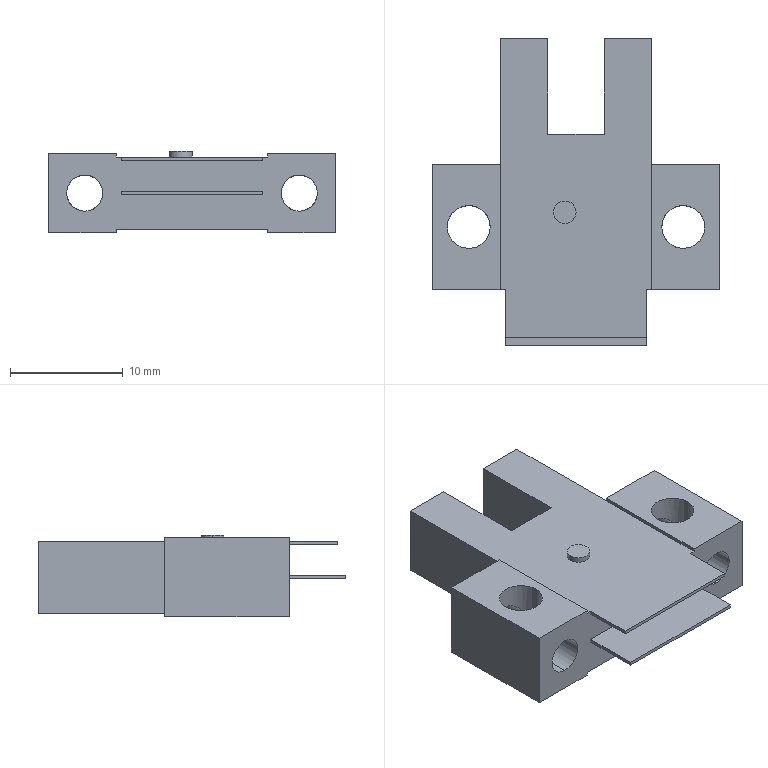Part | STEP file | 0246_007_FPMK54 | 1 solid | 46 faces | box 25.4 x 27.2 x 7.2 mm | volume 2312 mm3 | plane 32 | cylinder 14 | commonest cylinder face diameters 3.2 x8 3.8 x4 2 x2